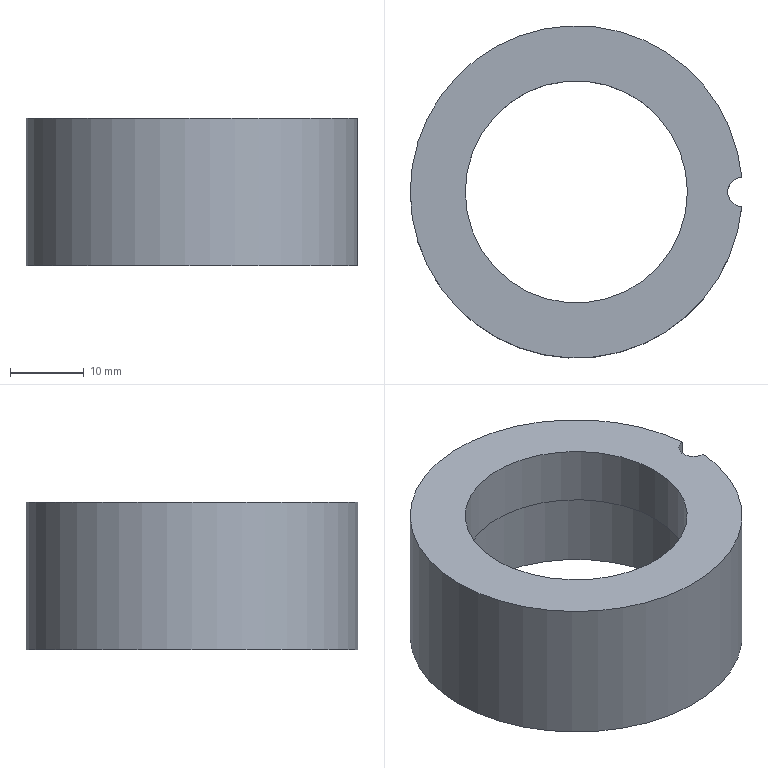Part | NX | features solid 2 | 1 solid | 7 faces | box 44.911 x 45 x 20 mm | volume 13778 mm3 | cylinder 4 | plane 3 | commonest cylinder face diameters 4 x1 30.1 x1 36 x1 45 x1
STEP:
#1=CARTESIAN_POINT('',(-222.546,-3.603,19.542));
#2=VERTEX_POINT('',#1);
#3=CARTESIAN_POINT('',(-222.546,-3.603,39.542));
#4=VERTEX_POINT('',#3);
#5=CARTESIAN_POINT('',(-222.546,-3.603,29.542));
#6=DIRECTION('',(0.,0.,1.));
#7=VECTOR('',#6,1000.);
#8=LINE('',#5,#7);
#9=EDGE_CURVE('',#2,#4,#8,.T.);
#10=ORIENTED_EDGE('',*,*,#9,.T.);
#11=CARTESIAN_POINT('',(-222.546,0.3926,39.542));
#12=VERTEX_POINT('',#11);
#13=CARTESIAN_POINT('',(-244.957,-1.605,39.542));
#14=DIRECTION('',(0.,0.,-1.));
#15=DIRECTION('',(1.,0.,0.));
#16=AXIS2_PLACEMENT_3D('',#13,#14,#15);
#17=CIRCLE('',#16,22.5);
#18=EDGE_CURVE('',#4,#12,#17,.T.);
#19=ORIENTED_EDGE('',*,*,#18,.T.);
#20=CARTESIAN_POINT('',(-222.546,0.3926,19.542));
#21=VERTEX_POINT('',#20);
#22=CARTESIAN_POINT('',(-222.546,0.3926,29.542));
#23=DIRECTION('',(0.,0.,1.));
#24=VECTOR('',#23,1000.);
#25=LINE('',#22,#24);
#26=EDGE_CURVE('',#12,#21,#25,.F.);
#27=ORIENTED_EDGE('',*,*,#26,.T.);
#28=CARTESIAN_POINT('',(-244.957,-1.605,19.542));
#29=DIRECTION('',(0.,0.,-1.));
#30=DIRECTION('',(1.,0.,0.));
#31=AXIS2_PLACEMENT_3D('',#28,#29,#30);
#32=CIRCLE('',#31,22.5);
#33=EDGE_CURVE('',#2,#21,#32,.T.);
#34=ORIENTED_EDGE('',*,*,#33,.F.);
#35=EDGE_LOOP('',(#10,#19,#27,#34));
#36=FACE_BOUND('',#35,.T.);
#37=CARTESIAN_POINT('',(-244.957,-1.605,19.542));
#38=DIRECTION('',(0.,0.,1.));
#39=DIRECTION('',(1.,0.,0.));
#40=AXIS2_PLACEMENT_3D('',#37,#38,#39);
#41=CYLINDRICAL_SURFACE('',#40,22.5);
#42=ADVANCED_FACE('',(#36),#41,.T.);
#43=CARTESIAN_POINT('',(-226.957,-1.605,19.542));
#44=VERTEX_POINT('',#43);
#45=CARTESIAN_POINT('',(-244.957,-1.605,19.542));
#46=DIRECTION('',(0.,0.,-1.));
#47=DIRECTION('',(1.,0.,0.));
#48=AXIS2_PLACEMENT_3D('',#45,#46,#47);
#49=CIRCLE('',#48,18.);
#50=EDGE_CURVE('',#44,#44,#49,.T.);
#51=ORIENTED_EDGE('',*,*,#50,.F.);
#52=EDGE_LOOP('',(#51));
#53=FACE_BOUND('',#52,.T.);
#54=ORIENTED_EDGE('',*,*,#33,.T.);
#55=CARTESIAN_POINT('',(-222.457,-1.605,19.542));
#56=DIRECTION('',(0.,0.,-1.));
#57=DIRECTION('',(1.,0.,0.));
#58=AXIS2_PLACEMENT_3D('',#55,#56,#57);
#59=CIRCLE('',#58,2.);
#60=EDGE_CURVE('',#2,#21,#59,.T.);
#61=ORIENTED_EDGE('',*,*,#60,.F.);
#62=EDGE_LOOP('',(#54,#61));
#63=FACE_BOUND('',#62,.T.);
#64=CARTESIAN_POINT('',(-244.957,-1.605,19.542));
#65=DIRECTION('',(0.,0.,1.));
#66=DIRECTION('',(1.,0.,0.));
#67=AXIS2_PLACEMENT_3D('',#64,#65,#66);
#68=PLANE('',#67);
#69=ADVANCED_FACE('',(#53,#63),#68,.F.);
#70=CARTESIAN_POINT('',(-229.907,-1.605,39.542));
#71=VERTEX_POINT('',#70);
#72=CARTESIAN_POINT('',(-244.957,-1.605,39.542));
#73=DIRECTION('',(0.,0.,-1.));
#74=DIRECTION('',(1.,0.,0.));
#75=AXIS2_PLACEMENT_3D('',#72,#73,#74);
#76=CIRCLE('',#75,15.05);
#77=EDGE_CURVE('',#71,#71,#76,.T.);
#78=ORIENTED_EDGE('',*,*,#77,.T.);
#79=EDGE_LOOP('',(#78));
#80=FACE_BOUND('',#79,.T.);
#81=CARTESIAN_POINT('',(-222.457,-1.605,39.542));
#82=DIRECTION('',(0.,0.,-1.));
#83=DIRECTION('',(1.,0.,0.));
#84=AXIS2_PLACEMENT_3D('',#81,#82,#83);
#85=CIRCLE('',#84,2.);
#86=EDGE_CURVE('',#4,#12,#85,.T.);
#87=ORIENTED_EDGE('',*,*,#86,.T.);
#88=ORIENTED_EDGE('',*,*,#18,.F.);
#89=EDGE_LOOP('',(#87,#88));
#90=FACE_BOUND('',#89,.T.);
#91=CARTESIAN_POINT('',(-244.957,-1.605,39.542));
#92=DIRECTION('',(0.,0.,1.));
#93=DIRECTION('',(1.,0.,0.));
#94=AXIS2_PLACEMENT_3D('',#91,#92,#93);
#95=PLANE('',#94);
#96=ADVANCED_FACE('',(#80,#90),#95,.T.);
#97=ORIENTED_EDGE('',*,*,#50,.T.);
#98=EDGE_LOOP('',(#97));
#99=FACE_BOUND('',#98,.T.);
#100=CARTESIAN_POINT('',(-226.957,-1.605,31.542));
#101=VERTEX_POINT('',#100);
#102=CARTESIAN_POINT('',(-244.957,-1.605,31.542));
#103=DIRECTION('',(0.,0.,-1.));
#104=DIRECTION('',(1.,0.,0.));
#105=AXIS2_PLACEMENT_3D('',#102,#103,#104);
#106=CIRCLE('',#105,18.);
#107=EDGE_CURVE('',#101,#101,#106,.T.);
#108=ORIENTED_EDGE('',*,*,#107,.F.);
#109=EDGE_LOOP('',(#108));
#110=FACE_BOUND('',#109,.T.);
#111=CARTESIAN_POINT('',(-244.957,-1.605,19.542));
#112=DIRECTION('',(0.,0.,1.));
#113=DIRECTION('',(1.,0.,0.));
#114=AXIS2_PLACEMENT_3D('',#111,#112,#113);
#115=CYLINDRICAL_SURFACE('',#114,18.);
#116=ADVANCED_FACE('',(#99,#110),#115,.F.);
#117=CARTESIAN_POINT('',(-229.907,-1.605,31.542));
#118=VERTEX_POINT('',#117);
#119=CARTESIAN_POINT('',(-244.957,-1.605,31.542));
#120=DIRECTION('',(0.,0.,-1.));
#121=DIRECTION('',(1.,0.,0.));
#122=AXIS2_PLACEMENT_3D('',#119,#120,#121);
#123=CIRCLE('',#122,15.05);
#124=EDGE_CURVE('',#118,#118,#123,.T.);
#125=ORIENTED_EDGE('',*,*,#124,.F.);
#126=EDGE_LOOP('',(#125));
#127=FACE_BOUND('',#126,.T.);
#128=ORIENTED_EDGE('',*,*,#107,.T.);
#129=EDGE_LOOP('',(#128));
#130=FACE_BOUND('',#129,.T.);
#131=CARTESIAN_POINT('',(-244.957,-1.605,31.542));
#132=DIRECTION('',(0.,0.,1.));
#133=DIRECTION('',(1.,0.,0.));
#134=AXIS2_PLACEMENT_3D('',#131,#132,#133);
#135=PLANE('',#134);
#136=ADVANCED_FACE('',(#127,#130),#135,.F.);
#137=ORIENTED_EDGE('',*,*,#9,.F.);
#138=ORIENTED_EDGE('',*,*,#60,.T.);
#139=ORIENTED_EDGE('',*,*,#26,.F.);
#140=ORIENTED_EDGE('',*,*,#86,.F.);
#141=EDGE_LOOP('',(#137,#138,#139,#140));
#142=FACE_BOUND('',#141,.T.);
#143=CARTESIAN_POINT('',(-222.457,-1.605,19.542));
#144=DIRECTION('',(0.,0.,1.));
#145=DIRECTION('',(1.,0.,0.));
#146=AXIS2_PLACEMENT_3D('',#143,#144,#145);
#147=CYLINDRICAL_SURFACE('',#146,2.);
#148=ADVANCED_FACE('',(#142),#147,.F.);
#149=ORIENTED_EDGE('',*,*,#77,.F.);
#150=EDGE_LOOP('',(#149));
#151=FACE_BOUND('',#150,.T.);
#152=ORIENTED_EDGE('',*,*,#124,.T.);
#153=EDGE_LOOP('',(#152));
#154=FACE_BOUND('',#153,.T.);
#155=CARTESIAN_POINT('',(-244.957,-1.605,19.542));
#156=DIRECTION('',(0.,0.,1.));
#157=DIRECTION('',(1.,0.,0.));
#158=AXIS2_PLACEMENT_3D('',#155,#156,#157);
#159=CYLINDRICAL_SURFACE('',#158,15.05);
#160=ADVANCED_FACE('',(#151,#154),#159,.F.);
#161=CLOSED_SHELL('',(#42,#69,#96,#116,#136,#148,#160));
#162=MANIFOLD_SOLID_BREP('',#161);
#163=(LENGTH_UNIT()NAMED_UNIT(*)SI_UNIT(.MILLI.,.METRE.));
#164=UNCERTAINTY_MEASURE_WITH_UNIT(LENGTH_MEASURE(0.00001),#163,'','');
#165=(NAMED_UNIT(*)PLANE_ANGLE_UNIT()SI_UNIT($,.RADIAN.));
#166=(NAMED_UNIT(*)SI_UNIT($,.STERADIAN.)SOLID_ANGLE_UNIT());
#167=(GEOMETRIC_REPRESENTATION_CONTEXT(3)GLOBAL_UNCERTAINTY_ASSIGNED_CONTEXT((#164))GLOBAL_UNIT_ASSIGNED_CONTEXT((#163,#165,#166))REPRESENTATION_CONTEXT('',''));
#168=ADVANCED_BREP_SHAPE_REPRESENTATION('',(#162),#167);